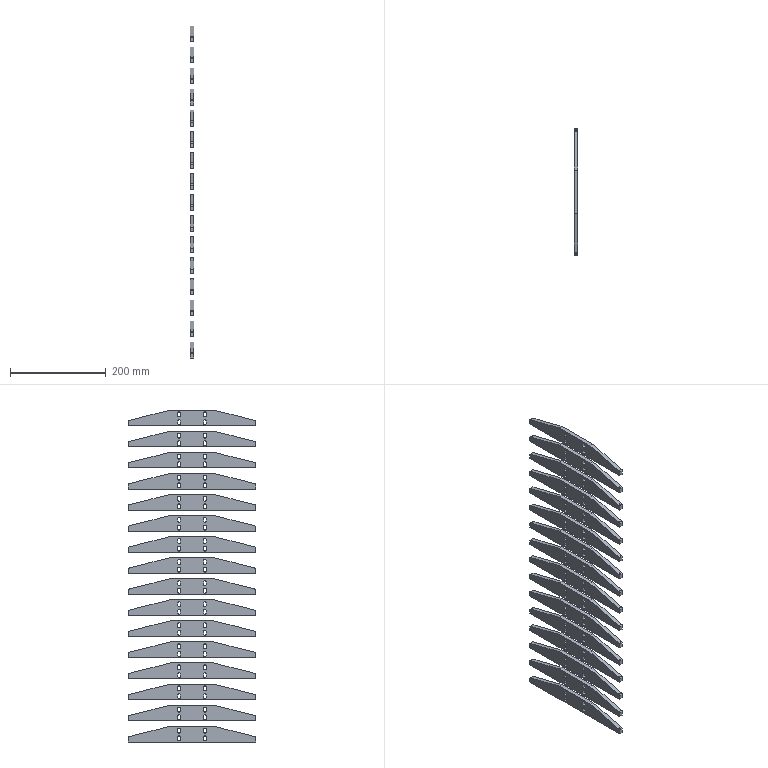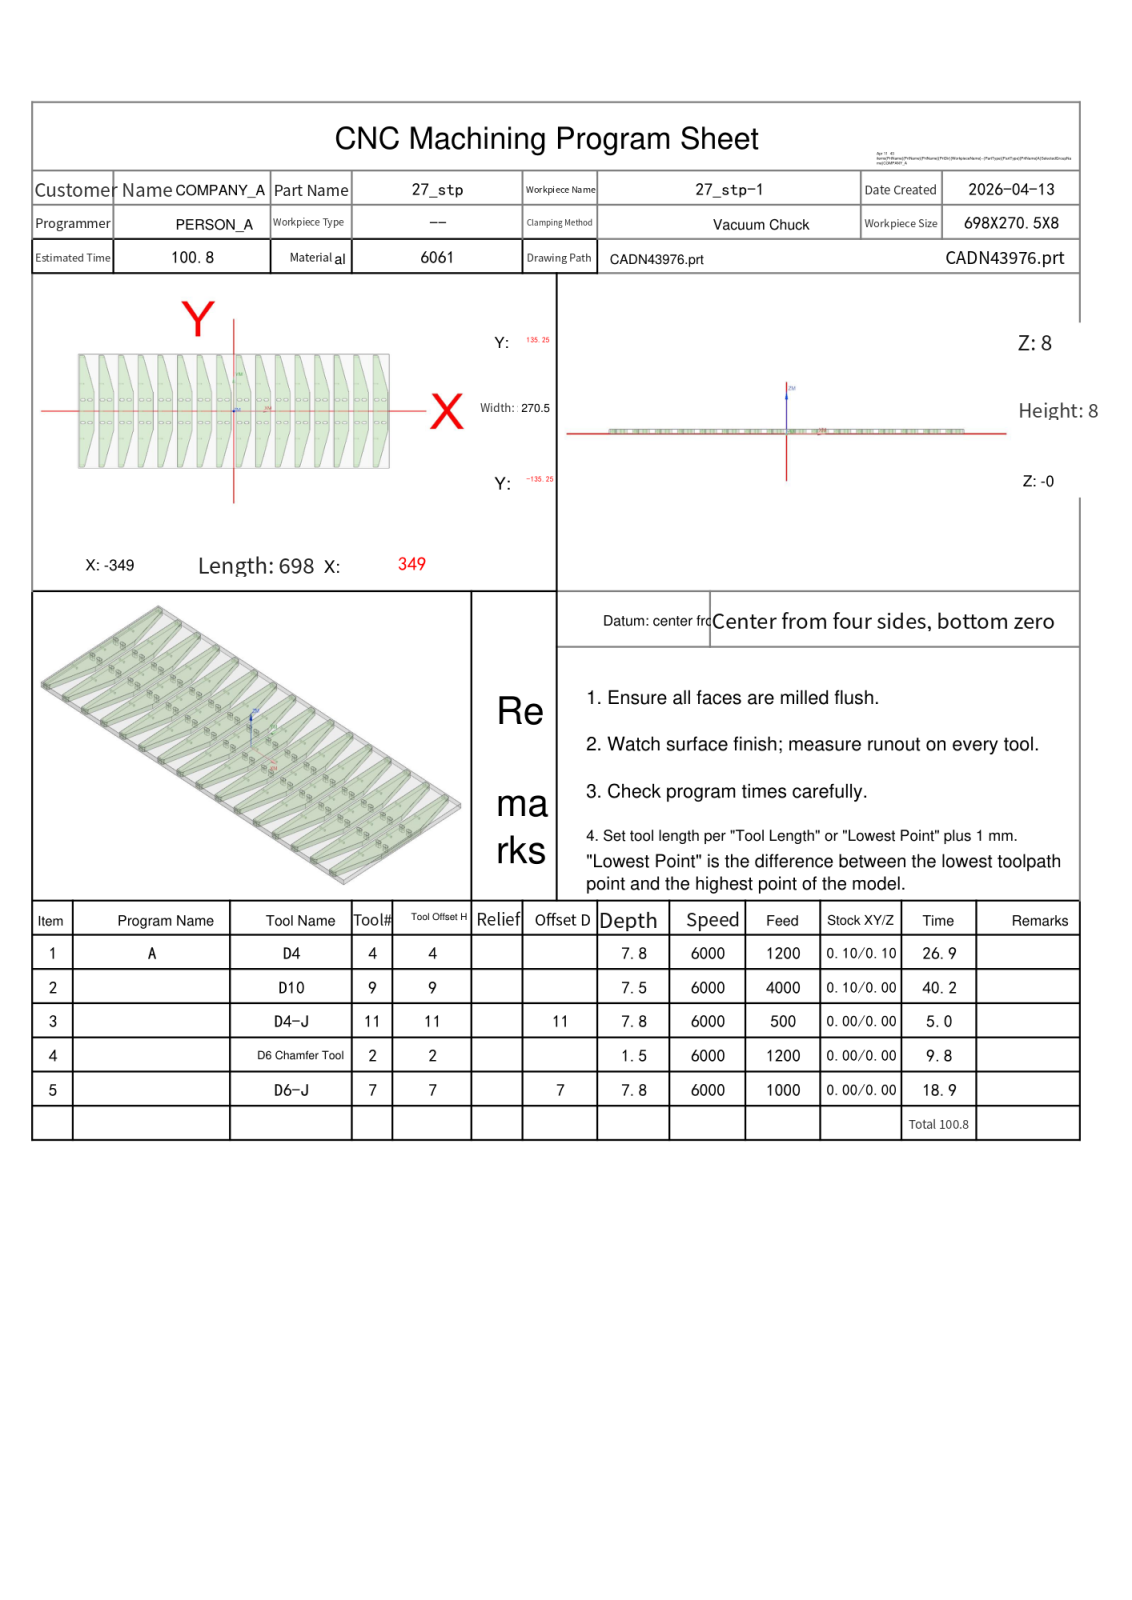NC program | NX | posted by the shop | part box 8 x 265.5 x 693 mm
Lines 1 to 837 of 21683:
%
O0001
(Machine time: 101.22 MIN)
(===Total Tool:5===)
(T4=D4      D=4.   R=0.   D-  H04 Z=0.2   )
(T9=D10     D=10.  R=0.   D-  H09 Z=0.5   )
(T11=D4-J   D=4.   R=0.   D11 H11 Z=0.2   )
(T2=D6 Chamfer Tool   D=6.   R=0.   D-  H02 Z=6.5   )
(T7=D6-J    D=6.   R=0.   D7  H07 Z=0.2   )
G80 G90 G17 G49 G40
G91 G28 Z0
M01
N1 T04 M06
(D4  D=4. R=0. H=04 ce=0.10 di=0.10)
G00 G90 G54 X-322.8 Y-26.35 M03 S6000
G43 H04 Z28.
M08
Z8.5
G01 X-325.3 Z8.457 F1200.
G03 X-325.95 Y-27. Z8.439 I0.0 J-.65
X-325.3 Y-27.65 Z8.421 I.65 J0.0
G01 X-320.3 Z8.335
G03 X-319.65 Y-27. Z8.317 I0.0 J.65
X-320.3 Y-26.35 Z8.299 I-.65 J0.0
G01 X-325.3 Z8.213
G03 X-325.95 Y-27. Z8.195 I0.0 J-.65
X-325.3 Y-27.65 Z8.177 I.65 J0.0
G01 X-320.3 Z8.09
G03 X-319.65 Y-27. Z8.073 I0.0 J.65
X-320.3 Y-26.35 Z8.055 I-.65 J0.0
G01 X-325.3 Z7.968
G03 X-325.95 Y-27. Z7.951 I0.0 J-.65
X-325.3 Y-27.65 Z7.933 I.65 J0.0
G01 X-320.3 Z7.846
G03 X-319.65 Y-27. Z7.829 I0.0 J.65
X-320.3 Y-26.35 Z7.811 I-.65 J0.0
G01 X-325.3 Z7.724
G03 X-325.95 Y-27. Z7.707 I0.0 J-.65
X-325.3 Y-27.65 Z7.689 I.65 J0.0
G01 X-320.3 Z7.602
G03 X-319.65 Y-27. Z7.585 I0.0 J.65
X-320.3 Y-26.35 Z7.567 I-.65 J0.0
G01 X-325.3 Z7.48
G03 X-325.95 Y-27. Z7.463 I0.0 J-.65
X-325.3 Y-27.65 Z7.445 I.65 J0.0
G01 X-320.3 Z7.358
G03 X-319.65 Y-27. Z7.34 I0.0 J.65
X-320.3 Y-26.35 Z7.323 I-.65 J0.0
G01 X-325.3 Z7.236
G03 X-325.95 Y-27. Z7.218 I0.0 J-.65
X-325.3 Y-27.65 Z7.201 I.65 J0.0
G01 X-320.3 Z7.114
G03 X-319.65 Y-27. Z7.096 I0.0 J.65
X-320.3 Y-26.35 Z7.079 I-.65 J0.0
G01 X-325.3 Z6.992
G03 X-325.95 Y-27. Z6.974 I0.0 J-.65
X-325.3 Y-27.65 Z6.957 I.65 J0.0
G01 X-320.3 Z6.87
G03 X-319.65 Y-27. Z6.852 I0.0 J.65
X-320.3 Y-26.35 Z6.835 I-.65 J0.0
G01 X-325.3 Z6.748
G03 X-325.95 Y-27. Z6.73 I0.0 J-.65
X-325.3 Y-27.65 Z6.712 I.65 J0.0
G01 X-320.3 Z6.626
G03 X-319.65 Y-27. Z6.608 I0.0 J.65
X-320.3 Y-26.35 Z6.59 I-.65 J0.0
G01 X-325.3 Z6.504
G03 X-325.95 Y-27. Z6.486 I0.0 J-.65
X-325.3 Y-27.65 Z6.468 I.65 J0.0
G01 X-320.3 Z6.382
G03 X-319.65 Y-27. Z6.364 I0.0 J.65
X-320.3 Y-26.35 Z6.346 I-.65 J0.0
G01 X-325.3 Z6.26
G03 X-325.95 Y-27. Z6.242 I0.0 J-.65
X-325.3 Y-27.65 Z6.224 I.65 J0.0
G01 X-320.3 Z6.138
G03 X-319.65 Y-27. Z6.12 I0.0 J.65
X-320.3 Y-26.35 Z6.102 I-.65 J0.0
G01 X-325.3 Z6.015
G03 X-325.95 Y-27. Z5.998 I0.0 J-.65
X-325.3 Y-27.65 Z5.98 I.65 J0.0
G01 X-320.3 Z5.893
G03 X-319.65 Y-27. Z5.876 I0.0 J.65
X-320.3 Y-26.35 Z5.858 I-.65 J0.0
G01 X-325.3 Z5.771
G03 X-325.95 Y-27. Z5.754 I0.0 J-.65
X-325.3 Y-27.65 Z5.736 I.65 J0.0
G01 X-320.3 Z5.649
G03 X-319.65 Y-27. Z5.632 I0.0 J.65
X-320.3 Y-26.35 Z5.614 I-.65 J0.0
G01 X-325.3 Z5.527
G03 X-325.95 Y-27. Z5.51 I0.0 J-.65
X-325.3 Y-27.65 Z5.492 I.65 J0.0
G01 X-320.3 Z5.405
G03 X-319.65 Y-27. Z5.388 I0.0 J.65
X-320.3 Y-26.35 Z5.37 I-.65 J0.0
G01 X-325.3 Z5.283
G03 X-325.95 Y-27. Z5.265 I0.0 J-.65
X-325.3 Y-27.65 Z5.248 I.65 J0.0
G01 X-320.3 Z5.161
G03 X-319.65 Y-27. Z5.143 I0.0 J.65
X-320.3 Y-26.35 Z5.126 I-.65 J0.0
G01 X-325.3 Z5.039
G03 X-325.95 Y-27. Z5.021 I0.0 J-.65
X-325.3 Y-27.65 Z5.004 I.65 J0.0
G01 X-320.3 Z4.917
G03 X-319.65 Y-27. Z4.899 I0.0 J.65
X-320.3 Y-26.35 Z4.882 I-.65 J0.0
G01 X-325.3 Z4.795
G03 X-325.95 Y-27. Z4.777 I0.0 J-.65
X-325.3 Y-27.65 Z4.76 I.65 J0.0
G01 X-320.3 Z4.673
G03 X-319.65 Y-27. Z4.655 I0.0 J.65
X-320.3 Y-26.35 Z4.637 I-.65 J0.0
G01 X-325.3 Z4.551
G03 X-325.95 Y-27. Z4.533 I0.0 J-.65
X-325.3 Y-27.65 Z4.515 I.65 J0.0
G01 X-320.3 Z4.429
G03 X-319.65 Y-27. Z4.411 I0.0 J.65
X-320.3 Y-26.35 Z4.393 I-.65 J0.0
G01 X-325.3 Z4.307
G03 X-325.95 Y-27. Z4.289 I0.0 J-.65
X-325.3 Y-27.65 Z4.271 I.65 J0.0
G01 X-320.3 Z4.185
G03 X-319.65 Y-27. Z4.167 I0.0 J.65
X-320.3 Y-26.35 Z4.149 I-.65 J0.0
G01 X-325.3 Z4.063
G03 X-325.95 Y-27. Z4.045 I0.0 J-.65
X-325.3 Y-27.65 Z4.027 I.65 J0.0
G01 X-320.3 Z3.94
G03 X-319.65 Y-27. Z3.923 I0.0 J.65
X-320.3 Y-26.35 Z3.905 I-.65 J0.0
G01 X-325.3 Z3.818
G03 X-325.95 Y-27. Z3.801 I0.0 J-.65
X-325.3 Y-27.65 Z3.783 I.65 J0.0
G01 X-320.3 Z3.696
G03 X-319.65 Y-27. Z3.679 I0.0 J.65
X-320.3 Y-26.35 Z3.661 I-.65 J0.0
G01 X-325.3 Z3.574
G03 X-325.95 Y-27. Z3.557 I0.0 J-.65
X-325.3 Y-27.65 Z3.539 I.65 J0.0
G01 X-320.3 Z3.452
G03 X-319.65 Y-27. Z3.435 I0.0 J.65
X-320.3 Y-26.35 Z3.417 I-.65 J0.0
G01 X-325.3 Z3.33
G03 X-325.95 Y-27. Z3.313 I0.0 J-.65
X-325.3 Y-27.65 Z3.295 I.65 J0.0
G01 X-320.3 Z3.208
G03 X-319.65 Y-27. Z3.19 I0.0 J.65
X-320.3 Y-26.35 Z3.173 I-.65 J0.0
G01 X-325.3 Z3.086
G03 X-325.95 Y-27. Z3.068 I0.0 J-.65
X-325.3 Y-27.65 Z3.051 I.65 J0.0
G01 X-320.3 Z2.964
G03 X-319.65 Y-27. Z2.946 I0.0 J.65
X-320.3 Y-26.35 Z2.929 I-.65 J0.0
G01 X-325.3 Z2.842
G03 X-325.95 Y-27. Z2.824 I0.0 J-.65
X-325.3 Y-27.65 Z2.807 I.65 J0.0
G01 X-320.3 Z2.72
G03 X-319.65 Y-27. Z2.702 I0.0 J.65
X-320.3 Y-26.35 Z2.685 I-.65 J0.0
G01 X-325.3 Z2.598
G03 X-325.95 Y-27. Z2.58 I0.0 J-.65
X-325.3 Y-27.65 Z2.562 I.65 J0.0
G01 X-320.3 Z2.476
G03 X-319.65 Y-27. Z2.458 I0.0 J.65
X-320.3 Y-26.35 Z2.44 I-.65 J0.0
G01 X-325.3 Z2.354
G03 X-325.95 Y-27. Z2.336 I0.0 J-.65
X-325.3 Y-27.65 Z2.318 I.65 J0.0
G01 X-320.3 Z2.232
G03 X-319.65 Y-27. Z2.214 I0.0 J.65
X-320.3 Y-26.35 Z2.196 I-.65 J0.0
G01 X-325.3 Z2.11
G03 X-325.95 Y-27. Z2.092 I0.0 J-.65
X-325.3 Y-27.65 Z2.074 I.65 J0.0
G01 X-320.3 Z1.988
G03 X-319.65 Y-27. Z1.97 I0.0 J.65
X-320.3 Y-26.35 Z1.952 I-.65 J0.0
G01 X-325.3 Z1.865
G03 X-325.95 Y-27. Z1.848 I0.0 J-.65
X-325.3 Y-27.65 Z1.83 I.65 J0.0
G01 X-320.3 Z1.743
G03 X-319.65 Y-27. Z1.726 I0.0 J.65
X-320.3 Y-26.35 Z1.708 I-.65 J0.0
G01 X-325.3 Z1.621
G03 X-325.95 Y-27. Z1.604 I0.0 J-.65
X-325.3 Y-27.65 Z1.586 I.65 J0.0
G01 X-320.3 Z1.499
G03 X-319.65 Y-27. Z1.482 I0.0 J.65
X-320.3 Y-26.35 Z1.464 I-.65 J0.0
G01 X-325.3 Z1.377
G03 X-325.95 Y-27. Z1.36 I0.0 J-.65
X-325.3 Y-27.65 Z1.342 I.65 J0.0
G01 X-320.3 Z1.255
G03 X-319.65 Y-27. Z1.238 I0.0 J.65
X-320.3 Y-26.35 Z1.22 I-.65 J0.0
G01 X-325.3 Z1.133
G03 X-325.95 Y-27. Z1.115 I0.0 J-.65
X-325.3 Y-27.65 Z1.098 I.65 J0.0
G01 X-320.3 Z1.011
G03 X-319.65 Y-27. Z.993 I0.0 J.65
X-320.3 Y-26.35 Z.976 I-.65 J0.0
G01 X-325.3 Z.889
G03 X-325.95 Y-27. Z.871 I0.0 J-.65
X-325.3 Y-27.65 Z.854 I.65 J0.0
G01 X-320.3 Z.767
G03 X-319.65 Y-27. Z.749 I0.0 J.65
X-320.3 Y-26.35 Z.732 I-.65 J0.0
G01 X-325.3 Z.645
G03 X-325.95 Y-27. Z.627 I0.0 J-.65
X-325.3 Y-27.65 Z.61 I.65 J0.0
G01 X-320.3 Z.523
G03 X-319.65 Y-27. Z.505 I0.0 J.65
X-320.3 Y-26.35 Z.487 I-.65 J0.0
G01 X-325.3 Z.401
G03 X-325.95 Y-27. Z.383 I0.0 J-.65
X-325.3 Y-27.65 Z.365 I.65 J0.0
G01 X-320.3 Z.279
G03 X-319.65 Y-27. Z.261 I0.0 J.65
X-320.3 Y-26.35 Z.243 I-.65 J0.0
G01 X-322.8 Z.2
X-325.3
G03 X-325.95 Y-27. I0.0 J-.65
X-325.3 Y-27.65 I.65 J0.0
G01 X-320.3
G03 X-319.65 Y-27. I0.0 J.65
X-320.3 Y-26.35 I-.65 J0.0
G01 X-322.8
X-323.3
Z1.2
G00 Z28.
X-338.8
Z8.5
G01 X-341.3 Z8.457
G03 X-341.95 Y-27. Z8.439 I0.0 J-.65
X-341.3 Y-27.65 Z8.421 I.65 J0.0
G01 X-336.3 Z8.335
G03 X-335.65 Y-27. Z8.317 I0.0 J.65
X-336.3 Y-26.35 Z8.299 I-.65 J0.0
G01 X-341.3 Z8.213
G03 X-341.95 Y-27. Z8.195 I0.0 J-.65
X-341.3 Y-27.65 Z8.177 I.65 J0.0
G01 X-336.3 Z8.09
G03 X-335.65 Y-27. Z8.073 I0.0 J.65
X-336.3 Y-26.35 Z8.055 I-.65 J0.0
G01 X-341.3 Z7.968
G03 X-341.95 Y-27. Z7.951 I0.0 J-.65
X-341.3 Y-27.65 Z7.933 I.65 J0.0
G01 X-336.3 Z7.846
G03 X-335.65 Y-27. Z7.829 I0.0 J.65
X-336.3 Y-26.35 Z7.811 I-.65 J0.0
G01 X-341.3 Z7.724
G03 X-341.95 Y-27. Z7.707 I0.0 J-.65
X-341.3 Y-27.65 Z7.689 I.65 J0.0
G01 X-336.3 Z7.602
G03 X-335.65 Y-27. Z7.585 I0.0 J.65
X-336.3 Y-26.35 Z7.567 I-.65 J0.0
G01 X-341.3 Z7.48
G03 X-341.95 Y-27. Z7.463 I0.0 J-.65
X-341.3 Y-27.65 Z7.445 I.65 J0.0
G01 X-336.3 Z7.358
G03 X-335.65 Y-27. Z7.34 I0.0 J.65
X-336.3 Y-26.35 Z7.323 I-.65 J0.0
G01 X-341.3 Z7.236
G03 X-341.95 Y-27. Z7.218 I0.0 J-.65
X-341.3 Y-27.65 Z7.201 I.65 J0.0
G01 X-336.3 Z7.114
G03 X-335.65 Y-27. Z7.096 I0.0 J.65
X-336.3 Y-26.35 Z7.079 I-.65 J0.0
G01 X-341.3 Z6.992
G03 X-341.95 Y-27. Z6.974 I0.0 J-.65
X-341.3 Y-27.65 Z6.957 I.65 J0.0
G01 X-336.3 Z6.87
G03 X-335.65 Y-27. Z6.852 I0.0 J.65
X-336.3 Y-26.35 Z6.835 I-.65 J0.0
G01 X-341.3 Z6.748
G03 X-341.95 Y-27. Z6.73 I0.0 J-.65
X-341.3 Y-27.65 Z6.712 I.65 J0.0
G01 X-336.3 Z6.626
G03 X-335.65 Y-27. Z6.608 I0.0 J.65
X-336.3 Y-26.35 Z6.59 I-.65 J0.0
G01 X-341.3 Z6.504
G03 X-341.95 Y-27. Z6.486 I0.0 J-.65
X-341.3 Y-27.65 Z6.468 I.65 J0.0
G01 X-336.3 Z6.382
G03 X-335.65 Y-27. Z6.364 I0.0 J.65
X-336.3 Y-26.35 Z6.346 I-.65 J0.0
G01 X-341.3 Z6.26
G03 X-341.95 Y-27. Z6.242 I0.0 J-.65
X-341.3 Y-27.65 Z6.224 I.65 J0.0
G01 X-336.3 Z6.138
G03 X-335.65 Y-27. Z6.12 I0.0 J.65
X-336.3 Y-26.35 Z6.102 I-.65 J0.0
G01 X-341.3 Z6.015
G03 X-341.95 Y-27. Z5.998 I0.0 J-.65
X-341.3 Y-27.65 Z5.98 I.65 J0.0
G01 X-336.3 Z5.893
G03 X-335.65 Y-27. Z5.876 I0.0 J.65
X-336.3 Y-26.35 Z5.858 I-.65 J0.0
G01 X-341.3 Z5.771
G03 X-341.95 Y-27. Z5.754 I0.0 J-.65
X-341.3 Y-27.65 Z5.736 I.65 J0.0
G01 X-336.3 Z5.649
G03 X-335.65 Y-27. Z5.632 I0.0 J.65
X-336.3 Y-26.35 Z5.614 I-.65 J0.0
G01 X-341.3 Z5.527
G03 X-341.95 Y-27. Z5.51 I0.0 J-.65
X-341.3 Y-27.65 Z5.492 I.65 J0.0
G01 X-336.3 Z5.405
G03 X-335.65 Y-27. Z5.388 I0.0 J.65
X-336.3 Y-26.35 Z5.37 I-.65 J0.0
G01 X-341.3 Z5.283
G03 X-341.95 Y-27. Z5.265 I0.0 J-.65
X-341.3 Y-27.65 Z5.248 I.65 J0.0
G01 X-336.3 Z5.161
G03 X-335.65 Y-27. Z5.143 I0.0 J.65
X-336.3 Y-26.35 Z5.126 I-.65 J0.0
G01 X-341.3 Z5.039
G03 X-341.95 Y-27. Z5.021 I0.0 J-.65
X-341.3 Y-27.65 Z5.004 I.65 J0.0
G01 X-336.3 Z4.917
G03 X-335.65 Y-27. Z4.899 I0.0 J.65
X-336.3 Y-26.35 Z4.882 I-.65 J0.0
G01 X-341.3 Z4.795
G03 X-341.95 Y-27. Z4.777 I0.0 J-.65
X-341.3 Y-27.65 Z4.76 I.65 J0.0
G01 X-336.3 Z4.673
G03 X-335.65 Y-27. Z4.655 I0.0 J.65
X-336.3 Y-26.35 Z4.637 I-.65 J0.0
G01 X-341.3 Z4.551
G03 X-341.95 Y-27. Z4.533 I0.0 J-.65
X-341.3 Y-27.65 Z4.515 I.65 J0.0
G01 X-336.3 Z4.429
G03 X-335.65 Y-27. Z4.411 I0.0 J.65
X-336.3 Y-26.35 Z4.393 I-.65 J0.0
G01 X-341.3 Z4.307
G03 X-341.95 Y-27. Z4.289 I0.0 J-.65
X-341.3 Y-27.65 Z4.271 I.65 J0.0
G01 X-336.3 Z4.185
G03 X-335.65 Y-27. Z4.167 I0.0 J.65
X-336.3 Y-26.35 Z4.149 I-.65 J0.0
G01 X-341.3 Z4.063
G03 X-341.95 Y-27. Z4.045 I0.0 J-.65
X-341.3 Y-27.65 Z4.027 I.65 J0.0
G01 X-336.3 Z3.94
G03 X-335.65 Y-27. Z3.923 I0.0 J.65
X-336.3 Y-26.35 Z3.905 I-.65 J0.0
G01 X-341.3 Z3.818
G03 X-341.95 Y-27. Z3.801 I0.0 J-.65
X-341.3 Y-27.65 Z3.783 I.65 J0.0
G01 X-336.3 Z3.696
G03 X-335.65 Y-27. Z3.679 I0.0 J.65
X-336.3 Y-26.35 Z3.661 I-.65 J0.0
G01 X-341.3 Z3.574
G03 X-341.95 Y-27. Z3.557 I0.0 J-.65
X-341.3 Y-27.65 Z3.539 I.65 J0.0
G01 X-336.3 Z3.452
G03 X-335.65 Y-27. Z3.435 I0.0 J.65
X-336.3 Y-26.35 Z3.417 I-.65 J0.0
G01 X-341.3 Z3.33
G03 X-341.95 Y-27. Z3.313 I0.0 J-.65
X-341.3 Y-27.65 Z3.295 I.65 J0.0
G01 X-336.3 Z3.208
G03 X-335.65 Y-27. Z3.19 I0.0 J.65
X-336.3 Y-26.35 Z3.173 I-.65 J0.0
G01 X-341.3 Z3.086
G03 X-341.95 Y-27. Z3.068 I0.0 J-.65
X-341.3 Y-27.65 Z3.051 I.65 J0.0
G01 X-336.3 Z2.964
G03 X-335.65 Y-27. Z2.946 I0.0 J.65
X-336.3 Y-26.35 Z2.929 I-.65 J0.0
G01 X-341.3 Z2.842
G03 X-341.95 Y-27. Z2.824 I0.0 J-.65
X-341.3 Y-27.65 Z2.807 I.65 J0.0
G01 X-336.3 Z2.72
G03 X-335.65 Y-27. Z2.702 I0.0 J.65
X-336.3 Y-26.35 Z2.685 I-.65 J0.0
G01 X-341.3 Z2.598
G03 X-341.95 Y-27. Z2.58 I0.0 J-.65
X-341.3 Y-27.65 Z2.562 I.65 J0.0
G01 X-336.3 Z2.476
G03 X-335.65 Y-27. Z2.458 I0.0 J.65
X-336.3 Y-26.35 Z2.44 I-.65 J0.0
G01 X-341.3 Z2.354
G03 X-341.95 Y-27. Z2.336 I0.0 J-.65
X-341.3 Y-27.65 Z2.318 I.65 J0.0
G01 X-336.3 Z2.232
G03 X-335.65 Y-27. Z2.214 I0.0 J.65
X-336.3 Y-26.35 Z2.196 I-.65 J0.0
G01 X-341.3 Z2.11
G03 X-341.95 Y-27. Z2.092 I0.0 J-.65
X-341.3 Y-27.65 Z2.074 I.65 J0.0
G01 X-336.3 Z1.988
G03 X-335.65 Y-27. Z1.97 I0.0 J.65
X-336.3 Y-26.35 Z1.952 I-.65 J0.0
G01 X-341.3 Z1.865
G03 X-341.95 Y-27. Z1.848 I0.0 J-.65
X-341.3 Y-27.65 Z1.83 I.65 J0.0
G01 X-336.3 Z1.743
G03 X-335.65 Y-27. Z1.726 I0.0 J.65
X-336.3 Y-26.35 Z1.708 I-.65 J0.0
G01 X-341.3 Z1.621
G03 X-341.95 Y-27. Z1.604 I0.0 J-.65
X-341.3 Y-27.65 Z1.586 I.65 J0.0
G01 X-336.3 Z1.499
G03 X-335.65 Y-27. Z1.482 I0.0 J.65
X-336.3 Y-26.35 Z1.464 I-.65 J0.0
G01 X-341.3 Z1.377
G03 X-341.95 Y-27. Z1.36 I0.0 J-.65
X-341.3 Y-27.65 Z1.342 I.65 J0.0
G01 X-336.3 Z1.255
G03 X-335.65 Y-27. Z1.238 I0.0 J.65
X-336.3 Y-26.35 Z1.22 I-.65 J0.0
G01 X-341.3 Z1.133
G03 X-341.95 Y-27. Z1.115 I0.0 J-.65
X-341.3 Y-27.65 Z1.098 I.65 J0.0
G01 X-336.3 Z1.011
G03 X-335.65 Y-27. Z.993 I0.0 J.65
X-336.3 Y-26.35 Z.976 I-.65 J0.0
G01 X-341.3 Z.889
G03 X-341.95 Y-27. Z.871 I0.0 J-.65
X-341.3 Y-27.65 Z.854 I.65 J0.0
G01 X-336.3 Z.767
G03 X-335.65 Y-27. Z.749 I0.0 J.65
X-336.3 Y-26.35 Z.732 I-.65 J0.0
G01 X-341.3 Z.645
G03 X-341.95 Y-27. Z.627 I0.0 J-.65
X-341.3 Y-27.65 Z.61 I.65 J0.0
G01 X-336.3 Z.523
G03 X-335.65 Y-27. Z.505 I0.0 J.65
X-336.3 Y-26.35 Z.487 I-.65 J0.0
G01 X-341.3 Z.401
G03 X-341.95 Y-27. Z.383 I0.0 J-.65
X-341.3 Y-27.65 Z.365 I.65 J0.0
G01 X-336.3 Z.279
G03 X-335.65 Y-27. Z.261 I0.0 J.65
X-336.3 Y-26.35 Z.243 I-.65 J0.0
G01 X-338.8 Z.2
X-341.3
G03 X-341.95 Y-27. I0.0 J-.65
X-341.3 Y-27.65 I.65 J0.0
G01 X-336.3
G03 X-335.65 Y-27. I0.0 J.65
X-336.3 Y-26.35 I-.65 J0.0
G01 X-338.8
X-339.3
Z1.2
G00 Z28.
X-278.8
Z8.5
G01 X-281.3 Z8.457
G03 X-281.95 Y-27. Z8.439 I0.0 J-.65
X-281.3 Y-27.65 Z8.421 I.65 J0.0
G01 X-276.3 Z8.335
G03 X-275.65 Y-27. Z8.317 I0.0 J.65
X-276.3 Y-26.35 Z8.299 I-.65 J0.0
G01 X-281.3 Z8.213
G03 X-281.95 Y-27. Z8.195 I0.0 J-.65
X-281.3 Y-27.65 Z8.177 I.65 J0.0
G01 X-276.3 Z8.09
G03 X-275.65 Y-27. Z8.073 I0.0 J.65
X-276.3 Y-26.35 Z8.055 I-.65 J0.0
G01 X-281.3 Z7.968
G03 X-281.95 Y-27. Z7.951 I0.0 J-.65
X-281.3 Y-27.65 Z7.933 I.65 J0.0
G01 X-276.3 Z7.846
G03 X-275.65 Y-27. Z7.829 I0.0 J.65
X-276.3 Y-26.35 Z7.811 I-.65 J0.0
G01 X-281.3 Z7.724
G03 X-281.95 Y-27. Z7.707 I0.0 J-.65
X-281.3 Y-27.65 Z7.689 I.65 J0.0
G01 X-276.3 Z7.602
G03 X-275.65 Y-27. Z7.585 I0.0 J.65
X-276.3 Y-26.35 Z7.567 I-.65 J0.0
G01 X-281.3 Z7.48
G03 X-281.95 Y-27. Z7.463 I0.0 J-.65
X-281.3 Y-27.65 Z7.445 I.65 J0.0
G01 X-276.3 Z7.358
G03 X-275.65 Y-27. Z7.34 I0.0 J.65
X-276.3 Y-26.35 Z7.323 I-.65 J0.0
G01 X-281.3 Z7.236
G03 X-281.95 Y-27. Z7.218 I0.0 J-.65
X-281.3 Y-27.65 Z7.201 I.65 J0.0
G01 X-276.3 Z7.114
G03 X-275.65 Y-27. Z7.096 I0.0 J.65
X-276.3 Y-26.35 Z7.079 I-.65 J0.0
G01 X-281.3 Z6.992
G03 X-281.95 Y-27. Z6.974 I0.0 J-.65
X-281.3 Y-27.65 Z6.957 I.65 J0.0
G01 X-276.3 Z6.87
G03 X-275.65 Y-27. Z6.852 I0.0 J.65
X-276.3 Y-26.35 Z6.835 I-.65 J0.0
G01 X-281.3 Z6.748
G03 X-281.95 Y-27. Z6.73 I0.0 J-.65
X-281.3 Y-27.65 Z6.712 I.65 J0.0
G01 X-276.3 Z6.626
G03 X-275.65 Y-27. Z6.608 I0.0 J.65
X-276.3 Y-26.35 Z6.59 I-.65 J0.0
G01 X-281.3 Z6.504
G03 X-281.95 Y-27. Z6.486 I0.0 J-.65
X-281.3 Y-27.65 Z6.468 I.65 J0.0
G01 X-276.3 Z6.382
G03 X-275.65 Y-27. Z6.364 I0.0 J.65
X-276.3 Y-26.35 Z6.346 I-.65 J0.0
G01 X-281.3 Z6.26
G03 X-281.95 Y-27. Z6.242 I0.0 J-.65
X-281.3 Y-27.65 Z6.224 I.65 J0.0
G01 X-276.3 Z6.138
G03 X-275.65 Y-27. Z6.12 I0.0 J.65
X-276.3 Y-26.35 Z6.102 I-.65 J0.0
G01 X-281.3 Z6.015
G03 X-281.95 Y-27. Z5.998 I0.0 J-.65
X-281.3 Y-27.65 Z5.98 I.65 J0.0
G01 X-276.3 Z5.893
G03 X-275.65 Y-27. Z5.876 I0.0 J.65
X-276.3 Y-26.35 Z5.858 I-.65 J0.0
G01 X-281.3 Z5.771
G03 X-281.95 Y-27. Z5.754 I0.0 J-.65
X-281.3 Y-27.65 Z5.736 I.65 J0.0
G01 X-276.3 Z5.649
G03 X-275.65 Y-27. Z5.632 I0.0 J.65
X-276.3 Y-26.35 Z5.614 I-.65 J0.0
G01 X-281.3 Z5.527
G03 X-281.95 Y-27. Z5.51 I0.0 J-.65
X-281.3 Y-27.65 Z5.492 I.65 J0.0
G01 X-276.3 Z5.405
G03 X-275.65 Y-27. Z5.388 I0.0 J.65
X-276.3 Y-26.35 Z5.37 I-.65 J0.0
G01 X-281.3 Z5.283
G03 X-281.95 Y-27. Z5.265 I0.0 J-.65
X-281.3 Y-27.65 Z5.248 I.65 J0.0
G01 X-276.3 Z5.161
G03 X-275.65 Y-27. Z5.143 I0.0 J.65
X-276.3 Y-26.35 Z5.126 I-.65 J0.0
G01 X-281.3 Z5.039
G03 X-281.95 Y-27. Z5.021 I0.0 J-.65
X-281.3 Y-27.65 Z5.004 I.65 J0.0
G01 X-276.3 Z4.917
G03 X-275.65 Y-27. Z4.899 I0.0 J.65
X-276.3 Y-26.35 Z4.882 I-.65 J0.0
G01 X-281.3 Z4.795
G03 X-281.95 Y-27. Z4.777 I0.0 J-.65
X-281.3 Y-27.65 Z4.76 I.65 J0.0
G01 X-276.3 Z4.673
G03 X-275.65 Y-27. Z4.655 I0.0 J.65
X-276.3 Y-26.35 Z4.637 I-.65 J0.0
G01 X-281.3 Z4.551
G03 X-281.95 Y-27. Z4.533 I0.0 J-.65
X-281.3 Y-27.65 Z4.515 I.65 J0.0
G01 X-276.3 Z4.429
G03 X-275.65 Y-27. Z4.411 I0.0 J.65
X-276.3 Y-26.35 Z4.393 I-.65 J0.0
G01 X-281.3 Z4.307
G03 X-281.95 Y-27. Z4.289 I0.0 J-.65
X-281.3 Y-27.65 Z4.271 I.65 J0.0
G01 X-276.3 Z4.185
G03 X-275.65 Y-27. Z4.167 I0.0 J.65
X-276.3 Y-26.35 Z4.149 I-.65 J0.0
G01 X-281.3 Z4.063
G03 X-281.95 Y-27. Z4.045 I0.0 J-.65
X-281.3 Y-27.65 Z4.027 I.65 J0.0
G01 X-276.3 Z3.94
G03 X-275.65 Y-27. Z3.923 I0.0 J.65
X-276.3 Y-26.35 Z3.905 I-.65 J0.0
G01 X-281.3 Z3.818
G03 X-281.95 Y-27. Z3.801 I0.0 J-.65
X-281.3 Y-27.65 Z3.783 I.65 J0.0
G01 X-276.3 Z3.696
G03 X-275.65 Y-27. Z3.679 I0.0 J.65
X-276.3 Y-26.35 Z3.661 I-.65 J0.0
G01 X-281.3 Z3.574
G03 X-281.95 Y-27. Z3.557 I0.0 J-.65
X-281.3 Y-27.65 Z3.539 I.65 J0.0
G01 X-276.3 Z3.452
G03 X-275.65 Y-27. Z3.435 I0.0 J.65
X-276.3 Y-26.35 Z3.417 I-.65 J0.0
G01 X-281.3 Z3.33
G03 X-281.95 Y-27. Z3.313 I0.0 J-.65
X-281.3 Y-27.65 Z3.295 I.65 J0.0
G01 X-276.3 Z3.208
G03 X-275.65 Y-27. Z3.19 I0.0 J.65
X-276.3 Y-26.35 Z3.173 I-.65 J0.0
G01 X-281.3 Z3.086
G03 X-281.95 Y-27. Z3.068 I0.0 J-.65
X-281.3 Y-27.65 Z3.051 I.65 J0.0
G01 X-276.3 Z2.964
G03 X-275.65 Y-27. Z2.946 I0.0 J.65
X-276.3 Y-26.35 Z2.929 I-.65 J0.0
G01 X-281.3 Z2.842
G03 X-281.95 Y-27. Z2.824 I0.0 J-.65
X-281.3 Y-27.65 Z2.807 I.65 J0.0
G01 X-276.3 Z2.72
G03 X-275.65 Y-27. Z2.702 I0.0 J.65
X-276.3 Y-26.35 Z2.685 I-.65 J0.0
G01 X-281.3 Z2.598
G03 X-281.95 Y-27. Z2.58 I0.0 J-.65
X-281.3 Y-27.65 Z2.562 I.65 J0.0
G01 X-276.3 Z2.476
G03 X-275.65 Y-27. Z2.458 I0.0 J.65
X-276.3 Y-26.35 Z2.44 I-.65 J0.0
G01 X-281.3 Z2.354
G03 X-281.95 Y-27. Z2.336 I0.0 J-.65
X-281.3 Y-27.65 Z2.318 I.65 J0.0
G01 X-276.3 Z2.232
G03 X-275.65 Y-27. Z2.214 I0.0 J.65
X-276.3 Y-26.35 Z2.196 I-.65 J0.0
G01 X-281.3 Z2.11
G03 X-281.95 Y-27. Z2.092 I0.0 J-.65
X-281.3 Y-27.65 Z2.074 I.65 J0.0
G01 X-276.3 Z1.988
G03 X-275.65 Y-27. Z1.97 I0.0 J.65
X-276.3 Y-26.35 Z1.952 I-.65 J0.0
G01 X-281.3 Z1.865
G03 X-281.95 Y-27. Z1.848 I0.0 J-.65
X-281.3 Y-27.65 Z1.83 I.65 J0.0
G01 X-276.3 Z1.743
G03 X-275.65 Y-27. Z1.726 I0.0 J.65
X-276.3 Y-26.35 Z1.708 I-.65 J0.0
G01 X-281.3 Z1.621
G03 X-281.95 Y-27. Z1.604 I0.0 J-.65
X-281.3 Y-27.65 Z1.586 I.65 J0.0
G01 X-276.3 Z1.499
G03 X-275.65 Y-27. Z1.482 I0.0 J.65
X-276.3 Y-26.35 Z1.464 I-.65 J0.0
G01 X-281.3 Z1.377
G03 X-281.95 Y-27. Z1.36 I0.0 J-.65
X-281.3 Y-27.65 Z1.342 I.65 J0.0
G01 X-276.3 Z1.255
G03 X-275.65 Y-27. Z1.238 I0.0 J.65
X-276.3 Y-26.35 Z1.22 I-.65 J0.0
G01 X-281.3 Z1.133
G03 X-281.95 Y-27. Z1.115 I0.0 J-.65
X-281.3 Y-27.65 Z1.098 I.65 J0.0
G01 X-276.3 Z1.011
G03 X-275.65 Y-27. Z.993 I0.0 J.65
X-276.3 Y-26.35 Z.976 I-.65 J0.0
G01 X-281.3 Z.889
G03 X-281.95 Y-27. Z.871 I0.0 J-.65
X-281.3 Y-27.65 Z.854 I.65 J0.0
G01 X-276.3 Z.767
G03 X-275.65 Y-27. Z.749 I0.0 J.65
X-276.3 Y-26.35 Z.732 I-.65 J0.0
G01 X-281.3 Z.645
G03 X-281.95 Y-27. Z.627 I0.0 J-.65
X-281.3 Y-27.65 Z.61 I.65 J0.0
G01 X-276.3 Z.523
G03 X-275.65 Y-27. Z.505 I0.0 J.65
X-276.3 Y-26.35 Z.487 I-.65 J0.0
G01 X-281.3 Z.401
G03 X-281.95 Y-27. Z.383 I0.0 J-.65
X-281.3 Y-27.65 Z.365 I.65 J0.0
G01 X-276.3 Z.279
G03 X-275.65 Y-27. Z.261 I0.0 J.65
X-276.3 Y-26.35 Z.243 I-.65 J0.0
G01 X-278.8 Z.2
X-281.3
G03 X-281.95 Y-27. I0.0 J-.65
X-281.3 Y-27.65 I.65 J0.0
G01 X-276.3
G03 X-275.65 Y-27. I0.0 J.65
X-276.3 Y-26.35 I-.65 J0.0
G01 X-278.8
X-279.3
Z1.2
G00 Z28.
X-294.8
Z8.5
G01 X-297.3 Z8.457
G03 X-297.95 Y-27. Z8.439 I0.0 J-.65
X-297.3 Y-27.65 Z8.421 I.65 J0.0
G01 X-292.3 Z8.335
G03 X-291.65 Y-27. Z8.317 I0.0 J.65
X-292.3 Y-26.35 Z8.299 I-.65 J0.0
G01 X-297.3 Z8.213
G03 X-297.95 Y-27. Z8.195 I0.0 J-.65
X-297.3 Y-27.65 Z8.177 I.65 J0.0
G01 X-292.3 Z8.09
G03 X-291.65 Y-27. Z8.073 I0.0 J.65
X-292.3 Y-26.35 Z8.055 I-.65 J0.0
G01 X-297.3 Z7.968
G03 X-297.95 Y-27. Z7.951 I0.0 J-.65
X-297.3 Y-27.65 Z7.933 I.65 J0.0
G01 X-292.3 Z7.846
G03 X-291.65 Y-27. Z7.829 I0.0 J.65
X-292.3 Y-26.35 Z7.811 I-.65 J0.0
G01 X-297.3 Z7.724
G03 X-297.95 Y-27. Z7.707 I0.0 J-.65
X-297.3 Y-27.65 Z7.689 I.65 J0.0
G01 X-292.3 Z7.602
G03 X-291.65 Y-27. Z7.585 I0.0 J.65
X-292.3 Y-26.35 Z7.567 I-.65 J0.0
G01 X-297.3 Z7.48
G03 X-297.95 Y-27. Z7.463 I0.0 J-.65
X-297.3 Y-27.65 Z7.445 I.65 J0.0
G01 X-292.3 Z7.358
G03 X-291.65 Y-27. Z7.34 I0.0 J.65
X-292.3 Y-26.35 Z7.323 I-.65 J0.0
G01 X-297.3 Z7.236
G03 X-297.95 Y-27. Z7.218 I0.0 J-.65
X-297.3 Y-27.65 Z7.201 I.65 J0.0
G01 X-292.3 Z7.114
G03 X-291.65 Y-27. Z7.096 I0.0 J.65
X-292.3 Y-26.35 Z7.079 I-.65 J0.0
G01 X-297.3 Z6.992
G03 X-297.95 Y-27. Z6.974 I0.0 J-.65
X-297.3 Y-27.65 Z6.957 I.65 J0.0
G01 X-292.3 Z6.87
G03 X-291.65 Y-27. Z6.852 I0.0 J.65
X-292.3 Y-26.35 Z6.835 I-.65 J0.0
G01 X-297.3 Z6.748
G03 X-297.95 Y-27. Z6.73 I0.0 J-.65
X-297.3 Y-27.65 Z6.712 I.65 J0.0
G01 X-292.3 Z6.626
G03 X-291.65 Y-27. Z6.608 I0.0 J.65
X-292.3 Y-26.35 Z6.59 I-.65 J0.0
G01 X-297.3 Z6.504
G03 X-297.95 Y-27. Z6.486 I0.0 J-.65
X-297.3 Y-27.65 Z6.468 I.65 J0.0
G01 X-292.3 Z6.382
G03 X-291.65 Y-27. Z6.364 I0.0 J.65
X-292.3 Y-26.35 Z6.346 I-.65 J0.0
G01 X-297.3 Z6.26
G03 X-297.95 Y-27. Z6.242 I0.0 J-.65
X-297.3 Y-27.65 Z6.224 I.65 J0.0
G01 X-292.3 Z6.138
G03 X-291.65 Y-27. Z6.12 I0.0 J.65
X-292.3 Y-26.35 Z6.102 I-.65 J0.0
G01 X-297.3 Z6.015
G03 X-297.95 Y-27. Z5.998 I0.0 J-.65
X-297.3 Y-27.65 Z5.98 I.65 J0.0
G01 X-292.3 Z5.893
G03 X-291.65 Y-27. Z5.876 I0.0 J.65
X-292.3 Y-26.35 Z5.858 I-.65 J0.0
G01 X-297.3 Z5.771
G03 X-297.95 Y-27. Z5.754 I0.0 J-.65
X-297.3 Y-27.65 Z5.736 I.65 J0.0
G01 X-292.3 Z5.649
G03 X-291.65 Y-27. Z5.632 I0.0 J.65
X-292.3 Y-26.35 Z5.614 I-.65 J0.0
G01 X-297.3 Z5.527
G03 X-297.95 Y-27. Z5.51 I0.0 J-.65
X-297.3 Y-27.65 Z5.492 I.65 J0.0
G01 X-292.3 Z5.405
G03 X-291.65 Y-27. Z5.388 I0.0 J.65
X-292.3 Y-26.35 Z5.37 I-.65 J0.0
G01 X-297.3 Z5.283
G03 X-297.95 Y-27. Z5.265 I0.0 J-.65
X-297.3 Y-27.65 Z5.248 I.65 J0.0
G01 X-292.3 Z5.161
G03 X-291.65 Y-27. Z5.143 I0.0 J.65
X-292.3 Y-26.35 Z5.126 I-.65 J0.0
G01 X-297.3 Z5.039
G03 X-297.95 Y-27. Z5.021 I0.0 J-.65
X-297.3 Y-27.65 Z5.004 I.65 J0.0
G01 X-292.3 Z4.917
G03 X-291.65 Y-27. Z4.899 I0.0 J.65
X-292.3 Y-26.35 Z4.882 I-.65 J0.0
G01 X-297.3 Z4.795
G03 X-297.95 Y-27. Z4.777 I0.0 J-.65
X-297.3 Y-27.65 Z4.76 I.65 J0.0
G01 X-292.3 Z4.673
G03 X-291.65 Y-27. Z4.655 I0.0 J.65
X-292.3 Y-26.35 Z4.637 I-.65 J0.0
G01 X-297.3 Z4.551
G03 X-297.95 Y-27. Z4.533 I0.0 J-.65
X-297.3 Y-27.65 Z4.515 I.65 J0.0
G01 X-292.3 Z4.429
G03 X-291.65 Y-27. Z4.411 I0.0 J.65
X-292.3 Y-26.35 Z4.393 I-.65 J0.0
G01 X-297.3 Z4.307
G03 X-297.95 Y-27. Z4.289 I0.0 J-.65
X-297.3 Y-27.65 Z4.271 I.65 J0.0
G01 X-292.3 Z4.185
G03 X-291.65 Y-27. Z4.167 I0.0 J.65
X-292.3 Y-26.35 Z4.149 I-.65 J0.0
G01 X-297.3 Z4.063
G03 X-297.95 Y-27. Z4.045 I0.0 J-.65
X-297.3 Y-27.65 Z4.027 I.65 J0.0
G01 X-292.3 Z3.94
G03 X-291.65 Y-27. Z3.923 I0.0 J.65
X-292.3 Y-26.35 Z3.905 I-.65 J0.0
G01 X-297.3 Z3.818
G03 X-297.95 Y-27. Z3.801 I0.0 J-.65
X-297.3 Y-27.65 Z3.783 I.65 J0.0
G01 X-292.3 Z3.696
G03 X-291.65 Y-27. Z3.679 I0.0 J.65
X-292.3 Y-26.35 Z3.661 I-.65 J0.0
G01 X-297.3 Z3.574
G03 X-297.95 Y-27. Z3.557 I0.0 J-.65
X-297.3 Y-27.65 Z3.539 I.65 J0.0
G01 X-292.3 Z3.452
G03 X-291.65 Y-27. Z3.435 I0.0 J.65
X-292.3 Y-26.35 Z3.417 I-.65 J0.0
G01 X-297.3 Z3.33
G03 X-297.95 Y-27. Z3.313 I0.0 J-.65
X-297.3 Y-27.65 Z3.295 I.65 J0.0
G01 X-292.3 Z3.208
G03 X-291.65 Y-27. Z3.19 I0.0 J.65
X-292.3 Y-26.35 Z3.173 I-.65 J0.0
G01 X-297.3 Z3.086
G03 X-297.95 Y-27. Z3.068 I0.0 J-.65
X-297.3 Y-27.65 Z3.051 I.65 J0.0
G01 X-292.3 Z2.964
G03 X-291.65 Y-27. Z2.946 I0.0 J.65
X-292.3 Y-26.35 Z2.929 I-.65 J0.0
G01 X-297.3 Z2.842
G03 X-297.95 Y-27. Z2.824 I0.0 J-.65
X-297.3 Y-27.65 Z2.807 I.65 J0.0
G01 X-292.3 Z2.72
G03 X-291.65 Y-27. Z2.702 I0.0 J.65
X-292.3 Y-26.35 Z2.685 I-.65 J0.0
G01 X-297.3 Z2.598
G03 X-297.95 Y-27. Z2.58 I0.0 J-.65
X-297.3 Y-27.65 Z2.562 I.65 J0.0
G01 X-292.3 Z2.476
G03 X-291.65 Y-27. Z2.458 I0.0 J.65
X-292.3 Y-26.35 Z2.44 I-.65 J0.0
G01 X-297.3 Z2.354
G03 X-297.95 Y-27. Z2.336 I0.0 J-.65
X-297.3 Y-27.65 Z2.318 I.65 J0.0
G01 X-292.3 Z2.232
G03 X-291.65 Y-27. Z2.214 I0.0 J.65
X-292.3 Y-26.35 Z2.196 I-.65 J0.0
G01 X-297.3 Z2.11
G03 X-297.95 Y-27. Z2.092 I0.0 J-.65
X-297.3 Y-27.65 Z2.074 I.65 J0.0
G01 X-292.3 Z1.988
G03 X-291.65 Y-27. Z1.97 I0.0 J.65
X-292.3 Y-26.35 Z1.952 I-.65 J0.0
G01 X-297.3 Z1.865
G03 X-297.95 Y-27. Z1.848 I0.0 J-.65
X-297.3 Y-27.65 Z1.83 I.65 J0.0
G01 X-292.3 Z1.743